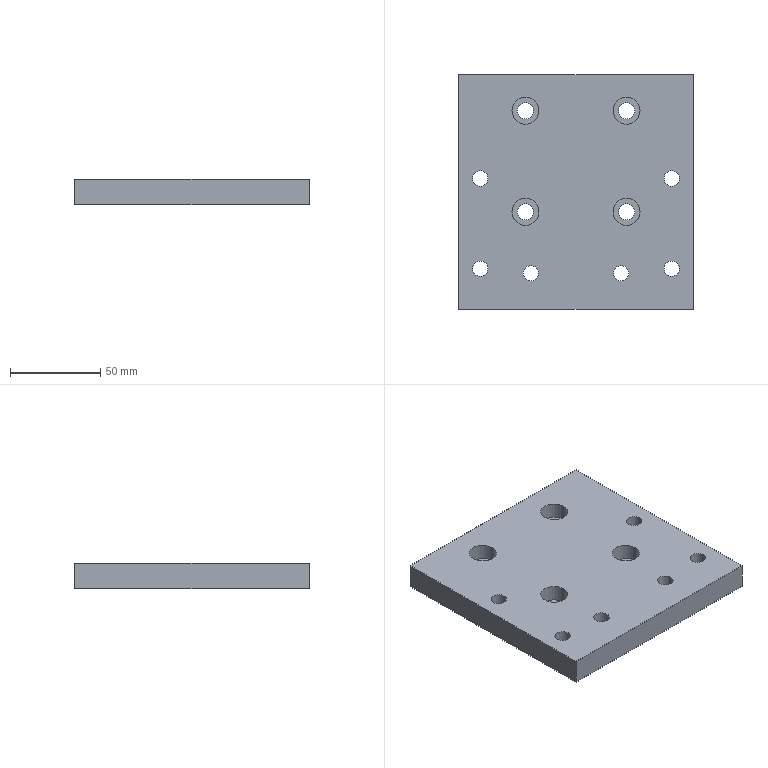Part | SolidWorks | features HoleWzd 3, Extrusion 1, ICE 1 | 1 solid | 38 faces | box 130 x 130 x 14 mm | volume 224199 mm3 | cylinder 28 | plane 10 | commonest cylinder face diameters 8.5 x12 9 x8 15 x8
STEP:
#1=CARTESIAN_POINT('',(122.25,72.5,14.));
#2=VERTEX_POINT('',#1);
#3=CARTESIAN_POINT('',(113.75,72.5,14.));
#4=VERTEX_POINT('',#3);
#5=CARTESIAN_POINT('',(118.,72.5,14.));
#6=DIRECTION('',(0.,0.,-1.));
#7=DIRECTION('',(-1.,0.,0.));
#8=AXIS2_PLACEMENT_3D('',#5,#6,#7);
#9=CIRCLE('',#8,4.25);
#10=EDGE_CURVE('',#2,#4,#9,.T.);
#11=ORIENTED_EDGE('',*,*,#10,.F.);
#12=CARTESIAN_POINT('',(122.25,72.5,0.));
#13=VERTEX_POINT('',#12);
#14=CARTESIAN_POINT('',(122.25,72.5,0.));
#15=DIRECTION('',(0.,0.,-1.));
#16=VECTOR('',#15,1000.);
#17=LINE('',#14,#16);
#18=EDGE_CURVE('',#2,#13,#17,.T.);
#19=ORIENTED_EDGE('',*,*,#18,.T.);
#20=CARTESIAN_POINT('',(113.75,72.5,0.));
#21=VERTEX_POINT('',#20);
#22=CARTESIAN_POINT('',(118.,72.5,0.));
#23=DIRECTION('',(0.,0.,-1.));
#24=DIRECTION('',(-1.,0.,0.));
#25=AXIS2_PLACEMENT_3D('',#22,#23,#24);
#26=CIRCLE('',#25,4.25);
#27=EDGE_CURVE('',#13,#21,#26,.T.);
#28=ORIENTED_EDGE('',*,*,#27,.T.);
#29=CARTESIAN_POINT('',(113.75,72.5,0.));
#30=DIRECTION('',(0.,0.,-1.));
#31=VECTOR('',#30,1000.);
#32=LINE('',#29,#31);
#33=EDGE_CURVE('',#4,#21,#32,.T.);
#34=ORIENTED_EDGE('',*,*,#33,.F.);
#35=EDGE_LOOP('',(#11,#19,#28,#34));
#36=FACE_OUTER_BOUND('',#35,.T.);
#37=CARTESIAN_POINT('',(118.,72.5,0.));
#38=DIRECTION('',(0.,0.,-1.));
#39=DIRECTION('',(-1.,0.,0.));
#40=AXIS2_PLACEMENT_3D('',#37,#38,#39);
#41=CYLINDRICAL_SURFACE('',#40,4.25);
#42=ADVANCED_FACE('',(#36),#41,.F.);
#43=CARTESIAN_POINT('',(122.25,22.5,14.));
#44=VERTEX_POINT('',#43);
#45=CARTESIAN_POINT('',(113.75,22.5,14.));
#46=VERTEX_POINT('',#45);
#47=CARTESIAN_POINT('',(118.,22.5,14.));
#48=DIRECTION('',(0.,0.,-1.));
#49=DIRECTION('',(-1.,0.,0.));
#50=AXIS2_PLACEMENT_3D('',#47,#48,#49);
#51=CIRCLE('',#50,4.25);
#52=EDGE_CURVE('',#44,#46,#51,.T.);
#53=ORIENTED_EDGE('',*,*,#52,.F.);
#54=CARTESIAN_POINT('',(122.25,22.5,0.));
#55=VERTEX_POINT('',#54);
#56=CARTESIAN_POINT('',(122.25,22.5,0.));
#57=DIRECTION('',(0.,0.,-1.));
#58=VECTOR('',#57,1000.);
#59=LINE('',#56,#58);
#60=EDGE_CURVE('',#44,#55,#59,.T.);
#61=ORIENTED_EDGE('',*,*,#60,.T.);
#62=CARTESIAN_POINT('',(113.75,22.5,0.));
#63=VERTEX_POINT('',#62);
#64=CARTESIAN_POINT('',(118.,22.5,0.));
#65=DIRECTION('',(0.,0.,-1.));
#66=DIRECTION('',(-1.,0.,0.));
#67=AXIS2_PLACEMENT_3D('',#64,#65,#66);
#68=CIRCLE('',#67,4.25);
#69=EDGE_CURVE('',#55,#63,#68,.T.);
#70=ORIENTED_EDGE('',*,*,#69,.T.);
#71=CARTESIAN_POINT('',(113.75,22.5,0.));
#72=DIRECTION('',(0.,0.,-1.));
#73=VECTOR('',#72,1000.);
#74=LINE('',#71,#73);
#75=EDGE_CURVE('',#46,#63,#74,.T.);
#76=ORIENTED_EDGE('',*,*,#75,.F.);
#77=EDGE_LOOP('',(#53,#61,#70,#76));
#78=FACE_OUTER_BOUND('',#77,.T.);
#79=CARTESIAN_POINT('',(118.,22.5,0.));
#80=DIRECTION('',(0.,0.,-1.));
#81=DIRECTION('',(-1.,0.,0.));
#82=AXIS2_PLACEMENT_3D('',#79,#80,#81);
#83=CYLINDRICAL_SURFACE('',#82,4.25);
#84=ADVANCED_FACE('',(#78),#83,.F.);
#85=CARTESIAN_POINT('',(16.25,72.5,14.));
#86=VERTEX_POINT('',#85);
#87=CARTESIAN_POINT('',(7.75,72.5,14.));
#88=VERTEX_POINT('',#87);
#89=CARTESIAN_POINT('',(12.,72.5,14.));
#90=DIRECTION('',(0.,0.,-1.));
#91=DIRECTION('',(-1.,0.,0.));
#92=AXIS2_PLACEMENT_3D('',#89,#90,#91);
#93=CIRCLE('',#92,4.25);
#94=EDGE_CURVE('',#86,#88,#93,.T.);
#95=ORIENTED_EDGE('',*,*,#94,.F.);
#96=CARTESIAN_POINT('',(16.25,72.5,0.));
#97=VERTEX_POINT('',#96);
#98=CARTESIAN_POINT('',(16.25,72.5,0.));
#99=DIRECTION('',(0.,0.,-1.));
#100=VECTOR('',#99,1000.);
#101=LINE('',#98,#100);
#102=EDGE_CURVE('',#86,#97,#101,.T.);
#103=ORIENTED_EDGE('',*,*,#102,.T.);
#104=CARTESIAN_POINT('',(7.75,72.5,0.));
#105=VERTEX_POINT('',#104);
#106=CARTESIAN_POINT('',(12.,72.5,0.));
#107=DIRECTION('',(0.,0.,-1.));
#108=DIRECTION('',(-1.,0.,0.));
#109=AXIS2_PLACEMENT_3D('',#106,#107,#108);
#110=CIRCLE('',#109,4.25);
#111=EDGE_CURVE('',#97,#105,#110,.T.);
#112=ORIENTED_EDGE('',*,*,#111,.T.);
#113=CARTESIAN_POINT('',(7.75,72.5,0.));
#114=DIRECTION('',(0.,0.,-1.));
#115=VECTOR('',#114,1000.);
#116=LINE('',#113,#115);
#117=EDGE_CURVE('',#88,#105,#116,.T.);
#118=ORIENTED_EDGE('',*,*,#117,.F.);
#119=EDGE_LOOP('',(#95,#103,#112,#118));
#120=FACE_OUTER_BOUND('',#119,.T.);
#121=CARTESIAN_POINT('',(12.,72.5,0.));
#122=DIRECTION('',(0.,0.,-1.));
#123=DIRECTION('',(-1.,0.,0.));
#124=AXIS2_PLACEMENT_3D('',#121,#122,#123);
#125=CYLINDRICAL_SURFACE('',#124,4.25);
#126=ADVANCED_FACE('',(#120),#125,.F.);
#127=CARTESIAN_POINT('',(16.25,22.5,14.));
#128=VERTEX_POINT('',#127);
#129=CARTESIAN_POINT('',(7.75,22.5,14.));
#130=VERTEX_POINT('',#129);
#131=CARTESIAN_POINT('',(12.,22.5,14.));
#132=DIRECTION('',(0.,0.,-1.));
#133=DIRECTION('',(-1.,0.,0.));
#134=AXIS2_PLACEMENT_3D('',#131,#132,#133);
#135=CIRCLE('',#134,4.25);
#136=EDGE_CURVE('',#128,#130,#135,.T.);
#137=ORIENTED_EDGE('',*,*,#136,.F.);
#138=CARTESIAN_POINT('',(16.25,22.5,0.));
#139=VERTEX_POINT('',#138);
#140=CARTESIAN_POINT('',(16.25,22.5,0.));
#141=DIRECTION('',(0.,0.,-1.));
#142=VECTOR('',#141,1000.);
#143=LINE('',#140,#142);
#144=EDGE_CURVE('',#128,#139,#143,.T.);
#145=ORIENTED_EDGE('',*,*,#144,.T.);
#146=CARTESIAN_POINT('',(7.75,22.5,0.));
#147=VERTEX_POINT('',#146);
#148=CARTESIAN_POINT('',(12.,22.5,0.));
#149=DIRECTION('',(0.,0.,-1.));
#150=DIRECTION('',(-1.,0.,0.));
#151=AXIS2_PLACEMENT_3D('',#148,#149,#150);
#152=CIRCLE('',#151,4.25);
#153=EDGE_CURVE('',#139,#147,#152,.T.);
#154=ORIENTED_EDGE('',*,*,#153,.T.);
#155=CARTESIAN_POINT('',(7.75,22.5,0.));
#156=DIRECTION('',(0.,0.,-1.));
#157=VECTOR('',#156,1000.);
#158=LINE('',#155,#157);
#159=EDGE_CURVE('',#130,#147,#158,.T.);
#160=ORIENTED_EDGE('',*,*,#159,.F.);
#161=EDGE_LOOP('',(#137,#145,#154,#160));
#162=FACE_OUTER_BOUND('',#161,.T.);
#163=CARTESIAN_POINT('',(12.,22.5,0.));
#164=DIRECTION('',(0.,0.,-1.));
#165=DIRECTION('',(-1.,0.,0.));
#166=AXIS2_PLACEMENT_3D('',#163,#164,#165);
#167=CYLINDRICAL_SURFACE('',#166,4.25);
#168=ADVANCED_FACE('',(#162),#167,.F.);
#169=CARTESIAN_POINT('',(94.25,20.,14.));
#170=VERTEX_POINT('',#169);
#171=CARTESIAN_POINT('',(85.75,20.,14.));
#172=VERTEX_POINT('',#171);
#173=CARTESIAN_POINT('',(90.,20.,14.));
#174=DIRECTION('',(0.,0.,-1.));
#175=DIRECTION('',(-1.,0.,0.));
#176=AXIS2_PLACEMENT_3D('',#173,#174,#175);
#177=CIRCLE('',#176,4.25);
#178=EDGE_CURVE('',#170,#172,#177,.T.);
#179=ORIENTED_EDGE('',*,*,#178,.F.);
#180=CARTESIAN_POINT('',(94.25,20.,0.));
#181=VERTEX_POINT('',#180);
#182=CARTESIAN_POINT('',(94.25,20.,0.));
#183=DIRECTION('',(0.,0.,-1.));
#184=VECTOR('',#183,1000.);
#185=LINE('',#182,#184);
#186=EDGE_CURVE('',#170,#181,#185,.T.);
#187=ORIENTED_EDGE('',*,*,#186,.T.);
#188=CARTESIAN_POINT('',(85.75,20.,0.));
#189=VERTEX_POINT('',#188);
#190=CARTESIAN_POINT('',(90.,20.,0.));
#191=DIRECTION('',(0.,0.,-1.));
#192=DIRECTION('',(-1.,0.,0.));
#193=AXIS2_PLACEMENT_3D('',#190,#191,#192);
#194=CIRCLE('',#193,4.25);
#195=EDGE_CURVE('',#181,#189,#194,.T.);
#196=ORIENTED_EDGE('',*,*,#195,.T.);
#197=CARTESIAN_POINT('',(85.75,20.,0.));
#198=DIRECTION('',(0.,0.,-1.));
#199=VECTOR('',#198,1000.);
#200=LINE('',#197,#199);
#201=EDGE_CURVE('',#172,#189,#200,.T.);
#202=ORIENTED_EDGE('',*,*,#201,.F.);
#203=EDGE_LOOP('',(#179,#187,#196,#202));
#204=FACE_OUTER_BOUND('',#203,.T.);
#205=CARTESIAN_POINT('',(90.,20.,0.));
#206=DIRECTION('',(0.,0.,-1.));
#207=DIRECTION('',(-1.,0.,0.));
#208=AXIS2_PLACEMENT_3D('',#205,#206,#207);
#209=CYLINDRICAL_SURFACE('',#208,4.25);
#210=ADVANCED_FACE('',(#204),#209,.F.);
#211=CARTESIAN_POINT('',(44.25,20.,14.));
#212=VERTEX_POINT('',#211);
#213=CARTESIAN_POINT('',(35.75,20.,14.));
#214=VERTEX_POINT('',#213);
#215=CARTESIAN_POINT('',(40.,20.,14.));
#216=DIRECTION('',(0.,0.,-1.));
#217=DIRECTION('',(-1.,0.,0.));
#218=AXIS2_PLACEMENT_3D('',#215,#216,#217);
#219=CIRCLE('',#218,4.25);
#220=EDGE_CURVE('',#212,#214,#219,.T.);
#221=ORIENTED_EDGE('',*,*,#220,.F.);
#222=CARTESIAN_POINT('',(44.25,20.,0.));
#223=VERTEX_POINT('',#222);
#224=CARTESIAN_POINT('',(44.25,20.,0.));
#225=DIRECTION('',(0.,0.,-1.));
#226=VECTOR('',#225,1000.);
#227=LINE('',#224,#226);
#228=EDGE_CURVE('',#212,#223,#227,.T.);
#229=ORIENTED_EDGE('',*,*,#228,.T.);
#230=CARTESIAN_POINT('',(35.75,20.,0.));
#231=VERTEX_POINT('',#230);
#232=CARTESIAN_POINT('',(40.,20.,0.));
#233=DIRECTION('',(0.,0.,-1.));
#234=DIRECTION('',(-1.,0.,0.));
#235=AXIS2_PLACEMENT_3D('',#232,#233,#234);
#236=CIRCLE('',#235,4.25);
#237=EDGE_CURVE('',#223,#231,#236,.T.);
#238=ORIENTED_EDGE('',*,*,#237,.T.);
#239=CARTESIAN_POINT('',(35.75,20.,0.));
#240=DIRECTION('',(0.,0.,-1.));
#241=VECTOR('',#240,1000.);
#242=LINE('',#239,#241);
#243=EDGE_CURVE('',#214,#231,#242,.T.);
#244=ORIENTED_EDGE('',*,*,#243,.F.);
#245=EDGE_LOOP('',(#221,#229,#238,#244));
#246=FACE_OUTER_BOUND('',#245,.T.);
#247=CARTESIAN_POINT('',(40.,20.,0.));
#248=DIRECTION('',(0.,0.,-1.));
#249=DIRECTION('',(-1.,0.,0.));
#250=AXIS2_PLACEMENT_3D('',#247,#248,#249);
#251=CYLINDRICAL_SURFACE('',#250,4.25);
#252=ADVANCED_FACE('',(#246),#251,.F.);
#253=CARTESIAN_POINT('',(29.5,110.,5.));
#254=VERTEX_POINT('',#253);
#255=CARTESIAN_POINT('',(44.5,110.,5.));
#256=VERTEX_POINT('',#255);
#257=CARTESIAN_POINT('',(37.,110.,5.));
#258=DIRECTION('',(0.,0.,1.));
#259=DIRECTION('',(1.,0.,0.));
#260=AXIS2_PLACEMENT_3D('',#257,#258,#259);
#261=CIRCLE('',#260,7.5);
#262=EDGE_CURVE('',#254,#256,#261,.T.);
#263=ORIENTED_EDGE('',*,*,#262,.F.);
#264=CARTESIAN_POINT('',(29.5,110.,14.));
#265=VERTEX_POINT('',#264);
#266=CARTESIAN_POINT('',(29.5,110.,14.));
#267=DIRECTION('',(0.,0.,1.));
#268=VECTOR('',#267,1000.);
#269=LINE('',#266,#268);
#270=EDGE_CURVE('',#254,#265,#269,.T.);
#271=ORIENTED_EDGE('',*,*,#270,.T.);
#272=CARTESIAN_POINT('',(44.5,110.,14.));
#273=VERTEX_POINT('',#272);
#274=CARTESIAN_POINT('',(37.,110.,14.));
#275=DIRECTION('',(0.,0.,1.));
#276=DIRECTION('',(1.,0.,0.));
#277=AXIS2_PLACEMENT_3D('',#274,#275,#276);
#278=CIRCLE('',#277,7.5);
#279=EDGE_CURVE('',#265,#273,#278,.T.);
#280=ORIENTED_EDGE('',*,*,#279,.T.);
#281=CARTESIAN_POINT('',(44.5,110.,14.));
#282=DIRECTION('',(0.,0.,1.));
#283=VECTOR('',#282,1000.);
#284=LINE('',#281,#283);
#285=EDGE_CURVE('',#256,#273,#284,.T.);
#286=ORIENTED_EDGE('',*,*,#285,.F.);
#287=EDGE_LOOP('',(#263,#271,#280,#286));
#288=FACE_OUTER_BOUND('',#287,.T.);
#289=CARTESIAN_POINT('',(37.,110.,14.));
#290=DIRECTION('',(0.,0.,1.));
#291=DIRECTION('',(1.,0.,0.));
#292=AXIS2_PLACEMENT_3D('',#289,#290,#291);
#293=CYLINDRICAL_SURFACE('',#292,7.5);
#294=ADVANCED_FACE('',(#288),#293,.F.);
#295=CARTESIAN_POINT('',(32.5,110.,0.));
#296=VERTEX_POINT('',#295);
#297=CARTESIAN_POINT('',(41.5,110.,0.));
#298=VERTEX_POINT('',#297);
#299=CARTESIAN_POINT('',(37.,110.,0.));
#300=DIRECTION('',(0.,0.,1.));
#301=DIRECTION('',(1.,0.,0.));
#302=AXIS2_PLACEMENT_3D('',#299,#300,#301);
#303=CIRCLE('',#302,4.5);
#304=EDGE_CURVE('',#296,#298,#303,.T.);
#305=ORIENTED_EDGE('',*,*,#304,.F.);
#306=CARTESIAN_POINT('',(32.5,110.,5.));
#307=VERTEX_POINT('',#306);
#308=CARTESIAN_POINT('',(32.5,110.,14.));
#309=DIRECTION('',(0.,0.,1.));
#310=VECTOR('',#309,1000.);
#311=LINE('',#308,#310);
#312=EDGE_CURVE('',#296,#307,#311,.T.);
#313=ORIENTED_EDGE('',*,*,#312,.T.);
#314=CARTESIAN_POINT('',(41.5,110.,5.));
#315=VERTEX_POINT('',#314);
#316=CARTESIAN_POINT('',(37.,110.,5.));
#317=DIRECTION('',(0.,0.,1.));
#318=DIRECTION('',(1.,0.,0.));
#319=AXIS2_PLACEMENT_3D('',#316,#317,#318);
#320=CIRCLE('',#319,4.5);
#321=EDGE_CURVE('',#307,#315,#320,.T.);
#322=ORIENTED_EDGE('',*,*,#321,.T.);
#323=CARTESIAN_POINT('',(41.5,110.,14.));
#324=DIRECTION('',(0.,0.,1.));
#325=VECTOR('',#324,1000.);
#326=LINE('',#323,#325);
#327=EDGE_CURVE('',#298,#315,#326,.T.);
#328=ORIENTED_EDGE('',*,*,#327,.F.);
#329=EDGE_LOOP('',(#305,#313,#322,#328));
#330=FACE_OUTER_BOUND('',#329,.T.);
#331=CARTESIAN_POINT('',(37.,110.,14.));
#332=DIRECTION('',(0.,0.,1.));
#333=DIRECTION('',(1.,0.,0.));
#334=AXIS2_PLACEMENT_3D('',#331,#332,#333);
#335=CYLINDRICAL_SURFACE('',#334,4.5);
#336=ADVANCED_FACE('',(#330),#335,.F.);
#337=CARTESIAN_POINT('',(85.5,110.,5.));
#338=VERTEX_POINT('',#337);
#339=CARTESIAN_POINT('',(100.5,110.,5.));
#340=VERTEX_POINT('',#339);
#341=CARTESIAN_POINT('',(93.,110.,5.));
#342=DIRECTION('',(0.,0.,1.));
#343=DIRECTION('',(1.,0.,0.));
#344=AXIS2_PLACEMENT_3D('',#341,#342,#343);
#345=CIRCLE('',#344,7.5);
#346=EDGE_CURVE('',#338,#340,#345,.T.);
#347=ORIENTED_EDGE('',*,*,#346,.F.);
#348=CARTESIAN_POINT('',(85.5,110.,14.));
#349=VERTEX_POINT('',#348);
#350=CARTESIAN_POINT('',(85.5,110.,14.));
#351=DIRECTION('',(0.,0.,1.));
#352=VECTOR('',#351,1000.);
#353=LINE('',#350,#352);
#354=EDGE_CURVE('',#338,#349,#353,.T.);
#355=ORIENTED_EDGE('',*,*,#354,.T.);
#356=CARTESIAN_POINT('',(100.5,110.,14.));
#357=VERTEX_POINT('',#356);
#358=CARTESIAN_POINT('',(93.,110.,14.));
#359=DIRECTION('',(0.,0.,1.));
#360=DIRECTION('',(1.,0.,0.));
#361=AXIS2_PLACEMENT_3D('',#358,#359,#360);
#362=CIRCLE('',#361,7.5);
#363=EDGE_CURVE('',#349,#357,#362,.T.);
#364=ORIENTED_EDGE('',*,*,#363,.T.);
#365=CARTESIAN_POINT('',(100.5,110.,14.));
#366=DIRECTION('',(0.,0.,1.));
#367=VECTOR('',#366,1000.);
#368=LINE('',#365,#367);
#369=EDGE_CURVE('',#340,#357,#368,.T.);
#370=ORIENTED_EDGE('',*,*,#369,.F.);
#371=EDGE_LOOP('',(#347,#355,#364,#370));
#372=FACE_OUTER_BOUND('',#371,.T.);
#373=CARTESIAN_POINT('',(93.,110.,14.));
#374=DIRECTION('',(0.,0.,1.));
#375=DIRECTION('',(1.,0.,0.));
#376=AXIS2_PLACEMENT_3D('',#373,#374,#375);
#377=CYLINDRICAL_SURFACE('',#376,7.5);
#378=ADVANCED_FACE('',(#372),#377,.F.);
#379=CARTESIAN_POINT('',(88.5,110.,0.));
#380=VERTEX_POINT('',#379);
#381=CARTESIAN_POINT('',(97.5,110.,0.));
#382=VERTEX_POINT('',#381);
#383=CARTESIAN_POINT('',(93.,110.,0.));
#384=DIRECTION('',(0.,0.,1.));
#385=DIRECTION('',(1.,0.,0.));
#386=AXIS2_PLACEMENT_3D('',#383,#384,#385);
#387=CIRCLE('',#386,4.5);
#388=EDGE_CURVE('',#380,#382,#387,.T.);
#389=ORIENTED_EDGE('',*,*,#388,.F.);
#390=CARTESIAN_POINT('',(88.5,110.,5.));
#391=VERTEX_POINT('',#390);
#392=CARTESIAN_POINT('',(88.5,110.,14.));
#393=DIRECTION('',(0.,0.,1.));
#394=VECTOR('',#393,1000.);
#395=LINE('',#392,#394);
#396=EDGE_CURVE('',#380,#391,#395,.T.);
#397=ORIENTED_EDGE('',*,*,#396,.T.);
#398=CARTESIAN_POINT('',(97.5,110.,5.));
#399=VERTEX_POINT('',#398);
#400=CARTESIAN_POINT('',(93.,110.,5.));
#401=DIRECTION('',(0.,0.,1.));
#402=DIRECTION('',(1.,0.,0.));
#403=AXIS2_PLACEMENT_3D('',#400,#401,#402);
#404=CIRCLE('',#403,4.5);
#405=EDGE_CURVE('',#391,#399,#404,.T.);
#406=ORIENTED_EDGE('',*,*,#405,.T.);
#407=CARTESIAN_POINT('',(97.5,110.,14.));
#408=DIRECTION('',(0.,0.,1.));
#409=VECTOR('',#408,1000.);
#410=LINE('',#407,#409);
#411=EDGE_CURVE('',#382,#399,#410,.T.);
#412=ORIENTED_EDGE('',*,*,#411,.F.);
#413=EDGE_LOOP('',(#389,#397,#406,#412));
#414=FACE_OUTER_BOUND('',#413,.T.);
#415=CARTESIAN_POINT('',(93.,110.,14.));
#416=DIRECTION('',(0.,0.,1.));
#417=DIRECTION('',(1.,0.,0.));
#418=AXIS2_PLACEMENT_3D('',#415,#416,#417);
#419=CYLINDRICAL_SURFACE('',#418,4.5);
#420=ADVANCED_FACE('',(#414),#419,.F.);
#421=CARTESIAN_POINT('',(85.5,54.,5.));
#422=VERTEX_POINT('',#421);
#423=CARTESIAN_POINT('',(100.5,54.,5.));
#424=VERTEX_POINT('',#423);
#425=CARTESIAN_POINT('',(93.,54.,5.));
#426=DIRECTION('',(0.,0.,1.));
#427=DIRECTION('',(1.,0.,0.));
#428=AXIS2_PLACEMENT_3D('',#425,#426,#427);
#429=CIRCLE('',#428,7.5);
#430=EDGE_CURVE('',#422,#424,#429,.T.);
#431=ORIENTED_EDGE('',*,*,#430,.F.);
#432=CARTESIAN_POINT('',(85.5,54.,14.));
#433=VERTEX_POINT('',#432);
#434=CARTESIAN_POINT('',(85.5,54.,14.));
#435=DIRECTION('',(0.,0.,1.));
#436=VECTOR('',#435,1000.);
#437=LINE('',#434,#436);
#438=EDGE_CURVE('',#422,#433,#437,.T.);
#439=ORIENTED_EDGE('',*,*,#438,.T.);
#440=CARTESIAN_POINT('',(100.5,54.,14.));
#441=VERTEX_POINT('',#440);
#442=CARTESIAN_POINT('',(93.,54.,14.));
#443=DIRECTION('',(0.,0.,1.));
#444=DIRECTION('',(1.,0.,0.));
#445=AXIS2_PLACEMENT_3D('',#442,#443,#444);
#446=CIRCLE('',#445,7.5);
#447=EDGE_CURVE('',#433,#441,#446,.T.);
#448=ORIENTED_EDGE('',*,*,#447,.T.);
#449=CARTESIAN_POINT('',(100.5,54.,14.));
#450=DIRECTION('',(0.,0.,1.));
#451=VECTOR('',#450,1000.);
#452=LINE('',#449,#451);
#453=EDGE_CURVE('',#424,#441,#452,.T.);
#454=ORIENTED_EDGE('',*,*,#453,.F.);
#455=EDGE_LOOP('',(#431,#439,#448,#454));
#456=FACE_OUTER_BOUND('',#455,.T.);
#457=CARTESIAN_POINT('',(93.,54.,14.));
#458=DIRECTION('',(0.,0.,1.));
#459=DIRECTION('',(1.,0.,0.));
#460=AXIS2_PLACEMENT_3D('',#457,#458,#459);
#461=CYLINDRICAL_SURFACE('',#460,7.5);
#462=ADVANCED_FACE('',(#456),#461,.F.);
#463=CARTESIAN_POINT('',(88.5,54.,0.));
#464=VERTEX_POINT('',#463);
#465=CARTESIAN_POINT('',(97.5,54.,0.));
#466=VERTEX_POINT('',#465);
#467=CARTESIAN_POINT('',(93.,54.,0.));
#468=DIRECTION('',(0.,0.,1.));
#469=DIRECTION('',(1.,0.,0.));
#470=AXIS2_PLACEMENT_3D('',#467,#468,#469);
#471=CIRCLE('',#470,4.5);
#472=EDGE_CURVE('',#464,#466,#471,.T.);
#473=ORIENTED_EDGE('',*,*,#472,.F.);
#474=CARTESIAN_POINT('',(88.5,54.,5.));
#475=VERTEX_POINT('',#474);
#476=CARTESIAN_POINT('',(88.5,54.,14.));
#477=DIRECTION('',(0.,0.,1.));
#478=VECTOR('',#477,1000.);
#479=LINE('',#476,#478);
#480=EDGE_CURVE('',#464,#475,#479,.T.);
#481=ORIENTED_EDGE('',*,*,#480,.T.);
#482=CARTESIAN_POINT('',(97.5,54.,5.));
#483=VERTEX_POINT('',#482);
#484=CARTESIAN_POINT('',(93.,54.,5.));
#485=DIRECTION('',(0.,0.,1.));
#486=DIRECTION('',(1.,0.,0.));
#487=AXIS2_PLACEMENT_3D('',#484,#485,#486);
#488=CIRCLE('',#487,4.5);
#489=EDGE_CURVE('',#475,#483,#488,.T.);
#490=ORIENTED_EDGE('',*,*,#489,.T.);
#491=CARTESIAN_POINT('',(97.5,54.,14.));
#492=DIRECTION('',(0.,0.,1.));
#493=VECTOR('',#492,1000.);
#494=LINE('',#491,#493);
#495=EDGE_CURVE('',#466,#483,#494,.T.);
#496=ORIENTED_EDGE('',*,*,#495,.F.);
#497=EDGE_LOOP('',(#473,#481,#490,#496));
#498=FACE_OUTER_BOUND('',#497,.T.);
#499=CARTESIAN_POINT('',(93.,54.,14.));
#500=DIRECTION('',(0.,0.,1.));
#501=DIRECTION('',(1.,0.,0.));
#502=AXIS2_PLACEMENT_3D('',#499,#500,#501);
#503=CYLINDRICAL_SURFACE('',#502,4.5);
#504=ADVANCED_FACE('',(#498),#503,.F.);
#505=CARTESIAN_POINT('',(29.5,54.,5.));
#506=VERTEX_POINT('',#505);
#507=CARTESIAN_POINT('',(44.5,54.,5.));
#508=VERTEX_POINT('',#507);
#509=CARTESIAN_POINT('',(37.,54.,5.));
#510=DIRECTION('',(0.,0.,1.));
#511=DIRECTION('',(1.,0.,0.));
#512=AXIS2_PLACEMENT_3D('',#509,#510,#511);
#513=CIRCLE('',#512,7.5);
#514=EDGE_CURVE('',#506,#508,#513,.T.);
#515=ORIENTED_EDGE('',*,*,#514,.F.);
#516=CARTESIAN_POINT('',(29.5,54.,14.));
#517=VERTEX_POINT('',#516);
#518=CARTESIAN_POINT('',(29.5,54.,14.));
#519=DIRECTION('',(0.,0.,1.));
#520=VECTOR('',#519,1000.);
#521=LINE('',#518,#520);
#522=EDGE_CURVE('',#506,#517,#521,.T.);
#523=ORIENTED_EDGE('',*,*,#522,.T.);
#524=CARTESIAN_POINT('',(44.5,54.,14.));
#525=VERTEX_POINT('',#524);
#526=CARTESIAN_POINT('',(37.,54.,14.));
#527=DIRECTION('',(0.,0.,1.));
#528=DIRECTION('',(1.,0.,0.));
#529=AXIS2_PLACEMENT_3D('',#526,#527,#528);
#530=CIRCLE('',#529,7.5);
#531=EDGE_CURVE('',#517,#525,#530,.T.);
#532=ORIENTED_EDGE('',*,*,#531,.T.);
#533=CARTESIAN_POINT('',(44.5,54.,14.));
#534=DIRECTION('',(0.,0.,1.));
#535=VECTOR('',#534,1000.);
#536=LINE('',#533,#535);
#537=EDGE_CURVE('',#508,#525,#536,.T.);
#538=ORIENTED_EDGE('',*,*,#537,.F.);
#539=EDGE_LOOP('',(#515,#523,#532,#538));
#540=FACE_OUTER_BOUND('',#539,.T.);
#541=CARTESIAN_POINT('',(37.,54.,14.));
#542=DIRECTION('',(0.,0.,1.));
#543=DIRECTION('',(1.,0.,0.));
#544=AXIS2_PLACEMENT_3D('',#541,#542,#543);
#545=CYLINDRICAL_SURFACE('',#544,7.5);
#546=ADVANCED_FACE('',(#540),#545,.F.);
#547=CARTESIAN_POINT('',(32.5,54.,0.));
#548=VERTEX_POINT('',#547);
#549=CARTESIAN_POINT('',(41.5,54.,0.));
#550=VERTEX_POINT('',#549);
#551=CARTESIAN_POINT('',(37.,54.,0.));
#552=DIRECTION('',(0.,0.,1.));
#553=DIRECTION('',(1.,0.,0.));
#554=AXIS2_PLACEMENT_3D('',#551,#552,#553);
#555=CIRCLE('',#554,4.5);
#556=EDGE_CURVE('',#548,#550,#555,.T.);
#557=ORIENTED_EDGE('',*,*,#556,.F.);
#558=CARTESIAN_POINT('',(32.5,54.,5.));
#559=VERTEX_POINT('',#558);
#560=CARTESIAN_POINT('',(32.5,54.,14.));
#561=DIRECTION('',(0.,0.,1.));
#562=VECTOR('',#561,1000.);
#563=LINE('',#560,#562);
#564=EDGE_CURVE('',#548,#559,#563,.T.);
#565=ORIENTED_EDGE('',*,*,#564,.T.);
#566=CARTESIAN_POINT('',(41.5,54.,5.));
#567=VERTEX_POINT('',#566);
#568=CARTESIAN_POINT('',(37.,54.,5.));
#569=DIRECTION('',(0.,0.,1.));
#570=DIRECTION('',(1.,0.,0.));
#571=AXIS2_PLACEMENT_3D('',#568,#569,#570);
#572=CIRCLE('',#571,4.5);
#573=EDGE_CURVE('',#559,#567,#572,.T.);
#574=ORIENTED_EDGE('',*,*,#573,.T.);
#575=CARTESIAN_POINT('',(41.5,54.,14.));
#576=DIRECTION('',(0.,0.,1.));
#577=VECTOR('',#576,1000.);
#578=LINE('',#575,#577);
#579=EDGE_CURVE('',#550,#567,#578,.T.);
#580=ORIENTED_EDGE('',*,*,#579,.F.);
#581=EDGE_LOOP('',(#557,#565,#574,#580));
#582=FACE_OUTER_BOUND('',#581,.T.);
#583=CARTESIAN_POINT('',(37.,54.,14.));
#584=DIRECTION('',(0.,0.,1.));
#585=DIRECTION('',(1.,0.,0.));
#586=AXIS2_PLACEMENT_3D('',#583,#584,#585);
#587=CYLINDRICAL_SURFACE('',#586,4.5);
#588=ADVANCED_FACE('',(#582),#587,.F.);
#589=CARTESIAN_POINT('',(0.,130.,0.));
#590=VERTEX_POINT('',#589);
#591=CARTESIAN_POINT('',(0.,0.,0.));
#592=VERTEX_POINT('',#591);
#593=CARTESIAN_POINT('',(0.,0.,0.));
#594=DIRECTION('',(0.,-1.,0.));
#595=VECTOR('',#594,1000.);
#596=LINE('',#593,#595);
#597=EDGE_CURVE('',#590,#592,#596,.T.);
#598=ORIENTED_EDGE('',*,*,#597,.T.);
#599=CARTESIAN_POINT('',(0.,0.,14.));
#600=VERTEX_POINT('',#599);
#601=CARTESIAN_POINT('',(0.,0.,14.));
#602=DIRECTION('',(0.,0.,-1.));
#603=VECTOR('',#602,1000.);
#604=LINE('',#601,#603);
#605=EDGE_CURVE('',#600,#592,#604,.T.);
#606=ORIENTED_EDGE('',*,*,#605,.F.);
#607=CARTESIAN_POINT('',(0.,130.,14.));
#608=VERTEX_POINT('',#607);
#609=CARTESIAN_POINT('',(0.,0.,14.));
#610=DIRECTION('',(0.,-1.,0.));
#611=VECTOR('',#610,1000.);
#612=LINE('',#609,#611);
#613=EDGE_CURVE('',#608,#600,#612,.T.);
#614=ORIENTED_EDGE('',*,*,#613,.F.);
#615=CARTESIAN_POINT('',(0.,130.,14.));
#616=DIRECTION('',(0.,0.,-1.));
#617=VECTOR('',#616,1000.);
#618=LINE('',#615,#617);
#619=EDGE_CURVE('',#608,#590,#618,.T.);
#620=ORIENTED_EDGE('',*,*,#619,.T.);
#621=EDGE_LOOP('',(#598,#606,#614,#620));
#622=FACE_OUTER_BOUND('',#621,.T.);
#623=CARTESIAN_POINT('',(0.,0.,14.));
#624=DIRECTION('',(1.,0.,0.));
#625=DIRECTION('',(0.,0.,-1.));
#626=AXIS2_PLACEMENT_3D('',#623,#624,#625);
#627=PLANE('',#626);
#628=ADVANCED_FACE('',(#622),#627,.F.);
#629=CARTESIAN_POINT('',(130.,0.,0.));
#630=VERTEX_POINT('',#629);
#631=CARTESIAN_POINT('',(0.,0.,0.));
#632=DIRECTION('',(1.,0.,0.));
#633=VECTOR('',#632,1000.);
#634=LINE('',#631,#633);
#635=EDGE_CURVE('',#592,#630,#634,.T.);
#636=ORIENTED_EDGE('',*,*,#635,.T.);
#637=CARTESIAN_POINT('',(130.,0.,14.));
#638=VERTEX_POINT('',#637);
#639=CARTESIAN_POINT('',(130.,0.,14.));
#640=DIRECTION('',(0.,0.,-1.));
#641=VECTOR('',#640,1000.);
#642=LINE('',#639,#641);
#643=EDGE_CURVE('',#638,#630,#642,.T.);
#644=ORIENTED_EDGE('',*,*,#643,.F.);
#645=CARTESIAN_POINT('',(0.,0.,14.));
#646=DIRECTION('',(1.,0.,0.));
#647=VECTOR('',#646,1000.);
#648=LINE('',#645,#647);
#649=EDGE_CURVE('',#600,#638,#648,.T.);
#650=ORIENTED_EDGE('',*,*,#649,.F.);
#651=ORIENTED_EDGE('',*,*,#605,.T.);
#652=EDGE_LOOP('',(#636,#644,#650,#651));
#653=FACE_OUTER_BOUND('',#652,.T.);
#654=CARTESIAN_POINT('',(0.,0.,14.));
#655=DIRECTION('',(0.,1.,0.));
#656=DIRECTION('',(0.,0.,1.));
#657=AXIS2_PLACEMENT_3D('',#654,#655,#656);
#658=PLANE('',#657);
#659=ADVANCED_FACE('',(#653),#658,.F.);
#660=CARTESIAN_POINT('',(130.,130.,0.));
#661=VERTEX_POINT('',#660);
#662=CARTESIAN_POINT('',(130.,0.,0.));
#663=DIRECTION('',(0.,1.,0.));
#664=VECTOR('',#663,1000.);
#665=LINE('',#662,#664);
#666=EDGE_CURVE('',#630,#661,#665,.T.);
#667=ORIENTED_EDGE('',*,*,#666,.T.);
#668=CARTESIAN_POINT('',(130.,130.,14.));
#669=VERTEX_POINT('',#668);
#670=CARTESIAN_POINT('',(130.,130.,14.));
#671=DIRECTION('',(0.,0.,-1.));
#672=VECTOR('',#671,1000.);
#673=LINE('',#670,#672);
#674=EDGE_CURVE('',#669,#661,#673,.T.);
#675=ORIENTED_EDGE('',*,*,#674,.F.);
#676=CARTESIAN_POINT('',(130.,0.,14.));
#677=DIRECTION('',(0.,1.,0.));
#678=VECTOR('',#677,1000.);
#679=LINE('',#676,#678);
#680=EDGE_CURVE('',#638,#669,#679,.T.);
#681=ORIENTED_EDGE('',*,*,#680,.F.);
#682=ORIENTED_EDGE('',*,*,#643,.T.);
#683=EDGE_LOOP('',(#667,#675,#681,#682));
#684=FACE_OUTER_BOUND('',#683,.T.);
#685=CARTESIAN_POINT('',(130.,0.,14.));
#686=DIRECTION('',(-1.,0.,0.));
#687=DIRECTION('',(0.,0.,1.));
#688=AXIS2_PLACEMENT_3D('',#685,#686,#687);
#689=PLANE('',#688);
#690=ADVANCED_FACE('',(#684),#689,.F.);
#691=CARTESIAN_POINT('',(0.,130.,0.));
#692=DIRECTION('',(-1.,0.,0.));
#693=VECTOR('',#692,1000.);
#694=LINE('',#691,#693);
#695=EDGE_CURVE('',#661,#590,#694,.T.);
#696=ORIENTED_EDGE('',*,*,#695,.T.);
#697=ORIENTED_EDGE('',*,*,#619,.F.);
#698=CARTESIAN_POINT('',(0.,130.,14.));
#699=DIRECTION('',(-1.,0.,0.));
#700=VECTOR('',#699,1000.);
#701=LINE('',#698,#700);
#702=EDGE_CURVE('',#669,#608,#701,.T.);
#703=ORIENTED_EDGE('',*,*,#702,.F.);
#704=ORIENTED_EDGE('',*,*,#674,.T.);
#705=EDGE_LOOP('',(#696,#697,#703,#704));
#706=FACE_OUTER_BOUND('',#705,.T.);
#707=CARTESIAN_POINT('',(0.,130.,14.));
#708=DIRECTION('',(0.,-1.,0.));
#709=DIRECTION('',(0.,0.,-1.));
#710=AXIS2_PLACEMENT_3D('',#707,#708,#709);
#711=PLANE('',#710);
#712=ADVANCED_FACE('',(#706),#711,.F.);
#713=CARTESIAN_POINT('',(118.,72.5,14.));
#714=DIRECTION('',(0.,0.,-1.));
#715=DIRECTION('',(-1.,0.,0.));
#716=AXIS2_PLACEMENT_3D('',#713,#714,#715);
#717=CIRCLE('',#716,4.25);
#718=EDGE_CURVE('',#4,#2,#717,.T.);
#719=ORIENTED_EDGE('',*,*,#718,.T.);
#720=ORIENTED_EDGE('',*,*,#10,.T.);
#721=EDGE_LOOP('',(#719,#720));
#722=FACE_BOUND('',#721,.T.);
#723=CARTESIAN_POINT('',(118.,22.5,14.));
#724=DIRECTION('',(0.,0.,-1.));
#725=DIRECTION('',(-1.,0.,0.));
#726=AXIS2_PLACEMENT_3D('',#723,#724,#725);
#727=CIRCLE('',#726,4.25);
#728=EDGE_CURVE('',#46,#44,#727,.T.);
#729=ORIENTED_EDGE('',*,*,#728,.T.);
#730=ORIENTED_EDGE('',*,*,#52,.T.);
#731=EDGE_LOOP('',(#729,#730));
#732=FACE_BOUND('',#731,.T.);
#733=CARTESIAN_POINT('',(12.,72.5,14.));
#734=DIRECTION('',(0.,0.,-1.));
#735=DIRECTION('',(-1.,0.,0.));
#736=AXIS2_PLACEMENT_3D('',#733,#734,#735);
#737=CIRCLE('',#736,4.25);
#738=EDGE_CURVE('',#88,#86,#737,.T.);
#739=ORIENTED_EDGE('',*,*,#738,.T.);
#740=ORIENTED_EDGE('',*,*,#94,.T.);
#741=EDGE_LOOP('',(#739,#740));
#742=FACE_BOUND('',#741,.T.);
#743=CARTESIAN_POINT('',(12.,22.5,14.));
#744=DIRECTION('',(0.,0.,-1.));
#745=DIRECTION('',(-1.,0.,0.));
#746=AXIS2_PLACEMENT_3D('',#743,#744,#745);
#747=CIRCLE('',#746,4.25);
#748=EDGE_CURVE('',#130,#128,#747,.T.);
#749=ORIENTED_EDGE('',*,*,#748,.T.);
#750=ORIENTED_EDGE('',*,*,#136,.T.);
#751=EDGE_LOOP('',(#749,#750));
#752=FACE_BOUND('',#751,.T.);
#753=CARTESIAN_POINT('',(90.,20.,14.));
#754=DIRECTION('',(0.,0.,-1.));
#755=DIRECTION('',(-1.,0.,0.));
#756=AXIS2_PLACEMENT_3D('',#753,#754,#755);
#757=CIRCLE('',#756,4.25);
#758=EDGE_CURVE('',#172,#170,#757,.T.);
#759=ORIENTED_EDGE('',*,*,#758,.T.);
#760=ORIENTED_EDGE('',*,*,#178,.T.);
#761=EDGE_LOOP('',(#759,#760));
#762=FACE_BOUND('',#761,.T.);
#763=CARTESIAN_POINT('',(40.,20.,14.));
#764=DIRECTION('',(0.,0.,-1.));
#765=DIRECTION('',(-1.,0.,0.));
#766=AXIS2_PLACEMENT_3D('',#763,#764,#765);
#767=CIRCLE('',#766,4.25);
#768=EDGE_CURVE('',#214,#212,#767,.T.);
#769=ORIENTED_EDGE('',*,*,#768,.T.);
#770=ORIENTED_EDGE('',*,*,#220,.T.);
#771=EDGE_LOOP('',(#769,#770));
#772=FACE_BOUND('',#771,.T.);
#773=CARTESIAN_POINT('',(37.,110.,14.));
#774=DIRECTION('',(0.,0.,1.));
#775=DIRECTION('',(1.,0.,0.));
#776=AXIS2_PLACEMENT_3D('',#773,#774,#775);
#777=CIRCLE('',#776,7.5);
#778=EDGE_CURVE('',#273,#265,#777,.T.);
#779=ORIENTED_EDGE('',*,*,#778,.F.);
#780=ORIENTED_EDGE('',*,*,#279,.F.);
#781=EDGE_LOOP('',(#779,#780));
#782=FACE_BOUND('',#781,.T.);
#783=CARTESIAN_POINT('',(93.,110.,14.));
#784=DIRECTION('',(0.,0.,1.));
#785=DIRECTION('',(1.,0.,0.));
#786=AXIS2_PLACEMENT_3D('',#783,#784,#785);
#787=CIRCLE('',#786,7.5);
#788=EDGE_CURVE('',#357,#349,#787,.T.);
#789=ORIENTED_EDGE('',*,*,#788,.F.);
#790=ORIENTED_EDGE('',*,*,#363,.F.);
#791=EDGE_LOOP('',(#789,#790));
#792=FACE_BOUND('',#791,.T.);
#793=CARTESIAN_POINT('',(93.,54.,14.));
#794=DIRECTION('',(0.,0.,1.));
#795=DIRECTION('',(1.,0.,0.));
#796=AXIS2_PLACEMENT_3D('',#793,#794,#795);
#797=CIRCLE('',#796,7.5);
#798=EDGE_CURVE('',#441,#433,#797,.T.);
#799=ORIENTED_EDGE('',*,*,#798,.F.);
#800=ORIENTED_EDGE('',*,*,#447,.F.);
#801=EDGE_LOOP('',(#799,#800));
#802=FACE_BOUND('',#801,.T.);
#803=CARTESIAN_POINT('',(37.,54.,14.));
#804=DIRECTION('',(0.,0.,1.));
#805=DIRECTION('',(1.,0.,0.));
#806=AXIS2_PLACEMENT_3D('',#803,#804,#805);
#807=CIRCLE('',#806,7.5);
#808=EDGE_CURVE('',#525,#517,#807,.T.);
#809=ORIENTED_EDGE('',*,*,#808,.F.);
#810=ORIENTED_EDGE('',*,*,#531,.F.);
#811=EDGE_LOOP('',(#809,#810));
#812=FACE_BOUND('',#811,.T.);
#813=ORIENTED_EDGE('',*,*,#613,.T.);
#814=ORIENTED_EDGE('',*,*,#649,.T.);
#815=ORIENTED_EDGE('',*,*,#680,.T.);
#816=ORIENTED_EDGE('',*,*,#702,.T.);
#817=EDGE_LOOP('',(#813,#814,#815,#816));
#818=FACE_OUTER_BOUND('',#817,.T.);
#819=CARTESIAN_POINT('',(0.,0.,14.));
#820=DIRECTION('',(0.,0.,-1.));
#821=DIRECTION('',(-1.,0.,0.));
#822=AXIS2_PLACEMENT_3D('',#819,#820,#821);
#823=PLANE('',#822);
#824=ADVANCED_FACE('',(#722,#732,#742,#752,#762,#772,#782,#792,#802,#812,#818),#823,.F.);
#825=CARTESIAN_POINT('',(118.,72.5,0.));
#826=DIRECTION('',(0.,0.,-1.));
#827=DIRECTION('',(-1.,0.,0.));
#828=AXIS2_PLACEMENT_3D('',#825,#826,#827);
#829=CIRCLE('',#828,4.25);
#830=EDGE_CURVE('',#21,#13,#829,.T.);
#831=ORIENTED_EDGE('',*,*,#830,.F.);
#832=ORIENTED_EDGE('',*,*,#27,.F.);
#833=EDGE_LOOP('',(#831,#832));
#834=FACE_BOUND('',#833,.T.);
#835=CARTESIAN_POINT('',(118.,22.5,0.));
#836=DIRECTION('',(0.,0.,-1.));
#837=DIRECTION('',(-1.,0.,0.));
#838=AXIS2_PLACEMENT_3D('',#835,#836,#837);
#839=CIRCLE('',#838,4.25);
#840=EDGE_CURVE('',#63,#55,#839,.T.);
#841=ORIENTED_EDGE('',*,*,#840,.F.);
#842=ORIENTED_EDGE('',*,*,#69,.F.);
#843=EDGE_LOOP('',(#841,#842));
#844=FACE_BOUND('',#843,.T.);
#845=CARTESIAN_POINT('',(12.,72.5,0.));
#846=DIRECTION('',(0.,0.,-1.));
#847=DIRECTION('',(-1.,0.,0.));
#848=AXIS2_PLACEMENT_3D('',#845,#846,#847);
#849=CIRCLE('',#848,4.25);
#850=EDGE_CURVE('',#105,#97,#849,.T.);
#851=ORIENTED_EDGE('',*,*,#850,.F.);
#852=ORIENTED_EDGE('',*,*,#111,.F.);
#853=EDGE_LOOP('',(#851,#852));
#854=FACE_BOUND('',#853,.T.);
#855=CARTESIAN_POINT('',(12.,22.5,0.));
#856=DIRECTION('',(0.,0.,-1.));
#857=DIRECTION('',(-1.,0.,0.));
#858=AXIS2_PLACEMENT_3D('',#855,#856,#857);
#859=CIRCLE('',#858,4.25);
#860=EDGE_CURVE('',#147,#139,#859,.T.);
#861=ORIENTED_EDGE('',*,*,#860,.F.);
#862=ORIENTED_EDGE('',*,*,#153,.F.);
#863=EDGE_LOOP('',(#861,#862));
#864=FACE_BOUND('',#863,.T.);
#865=CARTESIAN_POINT('',(90.,20.,0.));
#866=DIRECTION('',(0.,0.,-1.));
#867=DIRECTION('',(-1.,0.,0.));
#868=AXIS2_PLACEMENT_3D('',#865,#866,#867);
#869=CIRCLE('',#868,4.25);
#870=EDGE_CURVE('',#189,#181,#869,.T.);
#871=ORIENTED_EDGE('',*,*,#870,.F.);
#872=ORIENTED_EDGE('',*,*,#195,.F.);
#873=EDGE_LOOP('',(#871,#872));
#874=FACE_BOUND('',#873,.T.);
#875=CARTESIAN_POINT('',(40.,20.,0.));
#876=DIRECTION('',(0.,0.,-1.));
#877=DIRECTION('',(-1.,0.,0.));
#878=AXIS2_PLACEMENT_3D('',#875,#876,#877);
#879=CIRCLE('',#878,4.25);
#880=EDGE_CURVE('',#231,#223,#879,.T.);
#881=ORIENTED_EDGE('',*,*,#880,.F.);
#882=ORIENTED_EDGE('',*,*,#237,.F.);
#883=EDGE_LOOP('',(#881,#882));
#884=FACE_BOUND('',#883,.T.);
#885=CARTESIAN_POINT('',(37.,110.,0.));
#886=DIRECTION('',(0.,0.,1.));
#887=DIRECTION('',(1.,0.,0.));
#888=AXIS2_PLACEMENT_3D('',#885,#886,#887);
#889=CIRCLE('',#888,4.5);
#890=EDGE_CURVE('',#298,#296,#889,.T.);
#891=ORIENTED_EDGE('',*,*,#890,.T.);
#892=ORIENTED_EDGE('',*,*,#304,.T.);
#893=EDGE_LOOP('',(#891,#892));
#894=FACE_BOUND('',#893,.T.);
#895=CARTESIAN_POINT('',(93.,110.,0.));
#896=DIRECTION('',(0.,0.,1.));
#897=DIRECTION('',(1.,0.,0.));
#898=AXIS2_PLACEMENT_3D('',#895,#896,#897);
#899=CIRCLE('',#898,4.5);
#900=EDGE_CURVE('',#382,#380,#899,.T.);
#901=ORIENTED_EDGE('',*,*,#900,.T.);
#902=ORIENTED_EDGE('',*,*,#388,.T.);
#903=EDGE_LOOP('',(#901,#902));
#904=FACE_BOUND('',#903,.T.);
#905=CARTESIAN_POINT('',(93.,54.,0.));
#906=DIRECTION('',(0.,0.,1.));
#907=DIRECTION('',(1.,0.,0.));
#908=AXIS2_PLACEMENT_3D('',#905,#906,#907);
#909=CIRCLE('',#908,4.5);
#910=EDGE_CURVE('',#466,#464,#909,.T.);
#911=ORIENTED_EDGE('',*,*,#910,.T.);
#912=ORIENTED_EDGE('',*,*,#472,.T.);
#913=EDGE_LOOP('',(#911,#912));
#914=FACE_BOUND('',#913,.T.);
#915=CARTESIAN_POINT('',(37.,54.,0.));
#916=DIRECTION('',(0.,0.,1.));
#917=DIRECTION('',(1.,0.,0.));
#918=AXIS2_PLACEMENT_3D('',#915,#916,#917);
#919=CIRCLE('',#918,4.5);
#920=EDGE_CURVE('',#550,#548,#919,.T.);
#921=ORIENTED_EDGE('',*,*,#920,.T.);
#922=ORIENTED_EDGE('',*,*,#556,.T.);
#923=EDGE_LOOP('',(#921,#922));
#924=FACE_BOUND('',#923,.T.);
#925=ORIENTED_EDGE('',*,*,#597,.F.);
#926=ORIENTED_EDGE('',*,*,#695,.F.);
#927=ORIENTED_EDGE('',*,*,#666,.F.);
#928=ORIENTED_EDGE('',*,*,#635,.F.);
#929=EDGE_LOOP('',(#925,#926,#927,#928));
#930=FACE_OUTER_BOUND('',#929,.T.);
#931=CARTESIAN_POINT('',(0.,0.,0.));
#932=DIRECTION('',(0.,0.,-1.));
#933=DIRECTION('',(-1.,0.,0.));
#934=AXIS2_PLACEMENT_3D('',#931,#932,#933);
#935=PLANE('',#934);
#936=ADVANCED_FACE('',(#834,#844,#854,#864,#874,#884,#894,#904,#914,#924,#930),#935,.T.);
#937=ORIENTED_EDGE('',*,*,#564,.F.);
#938=ORIENTED_EDGE('',*,*,#920,.F.);
#939=ORIENTED_EDGE('',*,*,#579,.T.);
#940=CARTESIAN_POINT('',(37.,54.,5.));
#941=DIRECTION('',(0.,0.,1.));
#942=DIRECTION('',(1.,0.,0.));
#943=AXIS2_PLACEMENT_3D('',#940,#941,#942);
#944=CIRCLE('',#943,4.5);
#945=EDGE_CURVE('',#567,#559,#944,.T.);
#946=ORIENTED_EDGE('',*,*,#945,.T.);
#947=EDGE_LOOP('',(#937,#938,#939,#946));
#948=FACE_OUTER_BOUND('',#947,.T.);
#949=CARTESIAN_POINT('',(37.,54.,14.));
#950=DIRECTION('',(0.,0.,1.));
#951=DIRECTION('',(1.,0.,0.));
#952=AXIS2_PLACEMENT_3D('',#949,#950,#951);
#953=CYLINDRICAL_SURFACE('',#952,4.5);
#954=ADVANCED_FACE('',(#948),#953,.F.);
#955=ORIENTED_EDGE('',*,*,#945,.F.);
#956=ORIENTED_EDGE('',*,*,#573,.F.);
#957=EDGE_LOOP('',(#955,#956));
#958=FACE_BOUND('',#957,.T.);
#959=CARTESIAN_POINT('',(37.,54.,5.));
#960=DIRECTION('',(0.,0.,1.));
#961=DIRECTION('',(1.,0.,0.));
#962=AXIS2_PLACEMENT_3D('',#959,#960,#961);
#963=CIRCLE('',#962,7.5);
#964=EDGE_CURVE('',#508,#506,#963,.T.);
#965=ORIENTED_EDGE('',*,*,#964,.T.);
#966=ORIENTED_EDGE('',*,*,#514,.T.);
#967=EDGE_LOOP('',(#965,#966));
#968=FACE_OUTER_BOUND('',#967,.T.);
#969=CARTESIAN_POINT('',(41.5,54.,5.));
#970=DIRECTION('',(0.,0.,-1.));
#971=DIRECTION('',(-1.,0.,0.));
#972=AXIS2_PLACEMENT_3D('',#969,#970,#971);
#973=PLANE('',#972);
#974=ADVANCED_FACE('',(#958,#968),#973,.F.);
#975=ORIENTED_EDGE('',*,*,#522,.F.);
#976=ORIENTED_EDGE('',*,*,#964,.F.);
#977=ORIENTED_EDGE('',*,*,#537,.T.);
#978=ORIENTED_EDGE('',*,*,#808,.T.);
#979=EDGE_LOOP('',(#975,#976,#977,#978));
#980=FACE_OUTER_BOUND('',#979,.T.);
#981=CARTESIAN_POINT('',(37.,54.,14.));
#982=DIRECTION('',(0.,0.,1.));
#983=DIRECTION('',(1.,0.,0.));
#984=AXIS2_PLACEMENT_3D('',#981,#982,#983);
#985=CYLINDRICAL_SURFACE('',#984,7.5);
#986=ADVANCED_FACE('',(#980),#985,.F.);
#987=ORIENTED_EDGE('',*,*,#480,.F.);
#988=ORIENTED_EDGE('',*,*,#910,.F.);
#989=ORIENTED_EDGE('',*,*,#495,.T.);
#990=CARTESIAN_POINT('',(93.,54.,5.));
#991=DIRECTION('',(0.,0.,1.));
#992=DIRECTION('',(1.,0.,0.));
#993=AXIS2_PLACEMENT_3D('',#990,#991,#992);
#994=CIRCLE('',#993,4.5);
#995=EDGE_CURVE('',#483,#475,#994,.T.);
#996=ORIENTED_EDGE('',*,*,#995,.T.);
#997=EDGE_LOOP('',(#987,#988,#989,#996));
#998=FACE_OUTER_BOUND('',#997,.T.);
#999=CARTESIAN_POINT('',(93.,54.,14.));
#1000=DIRECTION('',(0.,0.,1.));
#1001=DIRECTION('',(1.,0.,0.));
#1002=AXIS2_PLACEMENT_3D('',#999,#1000,#1001);
#1003=CYLINDRICAL_SURFACE('',#1002,4.5);
#1004=ADVANCED_FACE('',(#998),#1003,.F.);
#1005=ORIENTED_EDGE('',*,*,#995,.F.);
#1006=ORIENTED_EDGE('',*,*,#489,.F.);
#1007=EDGE_LOOP('',(#1005,#1006));
#1008=FACE_BOUND('',#1007,.T.);
#1009=CARTESIAN_POINT('',(93.,54.,5.));
#1010=DIRECTION('',(0.,0.,1.));
#1011=DIRECTION('',(1.,0.,0.));
#1012=AXIS2_PLACEMENT_3D('',#1009,#1010,#1011);
#1013=CIRCLE('',#1012,7.5);
#1014=EDGE_CURVE('',#424,#422,#1013,.T.);
#1015=ORIENTED_EDGE('',*,*,#1014,.T.);
#1016=ORIENTED_EDGE('',*,*,#430,.T.);
#1017=EDGE_LOOP('',(#1015,#1016));
#1018=FACE_OUTER_BOUND('',#1017,.T.);
#1019=CARTESIAN_POINT('',(97.5,54.,5.));
#1020=DIRECTION('',(0.,0.,-1.));
#1021=DIRECTION('',(-1.,0.,0.));
#1022=AXIS2_PLACEMENT_3D('',#1019,#1020,#1021);
#1023=PLANE('',#1022);
#1024=ADVANCED_FACE('',(#1008,#1018),#1023,.F.);
#1025=ORIENTED_EDGE('',*,*,#438,.F.);
#1026=ORIENTED_EDGE('',*,*,#1014,.F.);
#1027=ORIENTED_EDGE('',*,*,#453,.T.);
#1028=ORIENTED_EDGE('',*,*,#798,.T.);
#1029=EDGE_LOOP('',(#1025,#1026,#1027,#1028));
#1030=FACE_OUTER_BOUND('',#1029,.T.);
#1031=CARTESIAN_POINT('',(93.,54.,14.));
#1032=DIRECTION('',(0.,0.,1.));
#1033=DIRECTION('',(1.,0.,0.));
#1034=AXIS2_PLACEMENT_3D('',#1031,#1032,#1033);
#1035=CYLINDRICAL_SURFACE('',#1034,7.5);
#1036=ADVANCED_FACE('',(#1030),#1035,.F.);
#1037=ORIENTED_EDGE('',*,*,#396,.F.);
#1038=ORIENTED_EDGE('',*,*,#900,.F.);
#1039=ORIENTED_EDGE('',*,*,#411,.T.);
#1040=CARTESIAN_POINT('',(93.,110.,5.));
#1041=DIRECTION('',(0.,0.,1.));
#1042=DIRECTION('',(1.,0.,0.));
#1043=AXIS2_PLACEMENT_3D('',#1040,#1041,#1042);
#1044=CIRCLE('',#1043,4.5);
#1045=EDGE_CURVE('',#399,#391,#1044,.T.);
#1046=ORIENTED_EDGE('',*,*,#1045,.T.);
#1047=EDGE_LOOP('',(#1037,#1038,#1039,#1046));
#1048=FACE_OUTER_BOUND('',#1047,.T.);
#1049=CARTESIAN_POINT('',(93.,110.,14.));
#1050=DIRECTION('',(0.,0.,1.));
#1051=DIRECTION('',(1.,0.,0.));
#1052=AXIS2_PLACEMENT_3D('',#1049,#1050,#1051);
#1053=CYLINDRICAL_SURFACE('',#1052,4.5);
#1054=ADVANCED_FACE('',(#1048),#1053,.F.);
#1055=ORIENTED_EDGE('',*,*,#1045,.F.);
#1056=ORIENTED_EDGE('',*,*,#405,.F.);
#1057=EDGE_LOOP('',(#1055,#1056));
#1058=FACE_BOUND('',#1057,.T.);
#1059=CARTESIAN_POINT('',(93.,110.,5.));
#1060=DIRECTION('',(0.,0.,1.));
#1061=DIRECTION('',(1.,0.,0.));
#1062=AXIS2_PLACEMENT_3D('',#1059,#1060,#1061);
#1063=CIRCLE('',#1062,7.5);
#1064=EDGE_CURVE('',#340,#338,#1063,.T.);
#1065=ORIENTED_EDGE('',*,*,#1064,.T.);
#1066=ORIENTED_EDGE('',*,*,#346,.T.);
#1067=EDGE_LOOP('',(#1065,#1066));
#1068=FACE_OUTER_BOUND('',#1067,.T.);
#1069=CARTESIAN_POINT('',(97.5,110.,5.));
#1070=DIRECTION('',(0.,0.,-1.));
#1071=DIRECTION('',(-1.,0.,0.));
#1072=AXIS2_PLACEMENT_3D('',#1069,#1070,#1071);
#1073=PLANE('',#1072);
#1074=ADVANCED_FACE('',(#1058,#1068),#1073,.F.);
#1075=ORIENTED_EDGE('',*,*,#354,.F.);
#1076=ORIENTED_EDGE('',*,*,#1064,.F.);
#1077=ORIENTED_EDGE('',*,*,#369,.T.);
#1078=ORIENTED_EDGE('',*,*,#788,.T.);
#1079=EDGE_LOOP('',(#1075,#1076,#1077,#1078));
#1080=FACE_OUTER_BOUND('',#1079,.T.);
#1081=CARTESIAN_POINT('',(93.,110.,14.));
#1082=DIRECTION('',(0.,0.,1.));
#1083=DIRECTION('',(1.,0.,0.));
#1084=AXIS2_PLACEMENT_3D('',#1081,#1082,#1083);
#1085=CYLINDRICAL_SURFACE('',#1084,7.5);
#1086=ADVANCED_FACE('',(#1080),#1085,.F.);
#1087=ORIENTED_EDGE('',*,*,#312,.F.);
#1088=ORIENTED_EDGE('',*,*,#890,.F.);
#1089=ORIENTED_EDGE('',*,*,#327,.T.);
#1090=CARTESIAN_POINT('',(37.,110.,5.));
#1091=DIRECTION('',(0.,0.,1.));
#1092=DIRECTION('',(1.,0.,0.));
#1093=AXIS2_PLACEMENT_3D('',#1090,#1091,#1092);
#1094=CIRCLE('',#1093,4.5);
#1095=EDGE_CURVE('',#315,#307,#1094,.T.);
#1096=ORIENTED_EDGE('',*,*,#1095,.T.);
#1097=EDGE_LOOP('',(#1087,#1088,#1089,#1096));
#1098=FACE_OUTER_BOUND('',#1097,.T.);
#1099=CARTESIAN_POINT('',(37.,110.,14.));
#1100=DIRECTION('',(0.,0.,1.));
#1101=DIRECTION('',(1.,0.,0.));
#1102=AXIS2_PLACEMENT_3D('',#1099,#1100,#1101);
#1103=CYLINDRICAL_SURFACE('',#1102,4.5);
#1104=ADVANCED_FACE('',(#1098),#1103,.F.);
#1105=ORIENTED_EDGE('',*,*,#1095,.F.);
#1106=ORIENTED_EDGE('',*,*,#321,.F.);
#1107=EDGE_LOOP('',(#1105,#1106));
#1108=FACE_BOUND('',#1107,.T.);
#1109=CARTESIAN_POINT('',(37.,110.,5.));
#1110=DIRECTION('',(0.,0.,1.));
#1111=DIRECTION('',(1.,0.,0.));
#1112=AXIS2_PLACEMENT_3D('',#1109,#1110,#1111);
#1113=CIRCLE('',#1112,7.5);
#1114=EDGE_CURVE('',#256,#254,#1113,.T.);
#1115=ORIENTED_EDGE('',*,*,#1114,.T.);
#1116=ORIENTED_EDGE('',*,*,#262,.T.);
#1117=EDGE_LOOP('',(#1115,#1116));
#1118=FACE_OUTER_BOUND('',#1117,.T.);
#1119=CARTESIAN_POINT('',(41.5,110.,5.));
#1120=DIRECTION('',(0.,0.,-1.));
#1121=DIRECTION('',(-1.,0.,0.));
#1122=AXIS2_PLACEMENT_3D('',#1119,#1120,#1121);
#1123=PLANE('',#1122);
#1124=ADVANCED_FACE('',(#1108,#1118),#1123,.F.);
#1125=ORIENTED_EDGE('',*,*,#270,.F.);
#1126=ORIENTED_EDGE('',*,*,#1114,.F.);
#1127=ORIENTED_EDGE('',*,*,#285,.T.);
#1128=ORIENTED_EDGE('',*,*,#778,.T.);
#1129=EDGE_LOOP('',(#1125,#1126,#1127,#1128));
#1130=FACE_OUTER_BOUND('',#1129,.T.);
#1131=CARTESIAN_POINT('',(37.,110.,14.));
#1132=DIRECTION('',(0.,0.,1.));
#1133=DIRECTION('',(1.,0.,0.));
#1134=AXIS2_PLACEMENT_3D('',#1131,#1132,#1133);
#1135=CYLINDRICAL_SURFACE('',#1134,7.5);
#1136=ADVANCED_FACE('',(#1130),#1135,.F.);
#1137=ORIENTED_EDGE('',*,*,#228,.F.);
#1138=ORIENTED_EDGE('',*,*,#768,.F.);
#1139=ORIENTED_EDGE('',*,*,#243,.T.);
#1140=ORIENTED_EDGE('',*,*,#880,.T.);
#1141=EDGE_LOOP('',(#1137,#1138,#1139,#1140));
#1142=FACE_OUTER_BOUND('',#1141,.T.);
#1143=CARTESIAN_POINT('',(40.,20.,0.));
#1144=DIRECTION('',(0.,0.,-1.));
#1145=DIRECTION('',(-1.,0.,0.));
#1146=AXIS2_PLACEMENT_3D('',#1143,#1144,#1145);
#1147=CYLINDRICAL_SURFACE('',#1146,4.25);
#1148=ADVANCED_FACE('',(#1142),#1147,.F.);
#1149=ORIENTED_EDGE('',*,*,#186,.F.);
#1150=ORIENTED_EDGE('',*,*,#758,.F.);
#1151=ORIENTED_EDGE('',*,*,#201,.T.);
#1152=ORIENTED_EDGE('',*,*,#870,.T.);
#1153=EDGE_LOOP('',(#1149,#1150,#1151,#1152));
#1154=FACE_OUTER_BOUND('',#1153,.T.);
#1155=CARTESIAN_POINT('',(90.,20.,0.));
#1156=DIRECTION('',(0.,0.,-1.));
#1157=DIRECTION('',(-1.,0.,0.));
#1158=AXIS2_PLACEMENT_3D('',#1155,#1156,#1157);
#1159=CYLINDRICAL_SURFACE('',#1158,4.25);
#1160=ADVANCED_FACE('',(#1154),#1159,.F.);
#1161=ORIENTED_EDGE('',*,*,#144,.F.);
#1162=ORIENTED_EDGE('',*,*,#748,.F.);
#1163=ORIENTED_EDGE('',*,*,#159,.T.);
#1164=ORIENTED_EDGE('',*,*,#860,.T.);
#1165=EDGE_LOOP('',(#1161,#1162,#1163,#1164));
#1166=FACE_OUTER_BOUND('',#1165,.T.);
#1167=CARTESIAN_POINT('',(12.,22.5,0.));
#1168=DIRECTION('',(0.,0.,-1.));
#1169=DIRECTION('',(-1.,0.,0.));
#1170=AXIS2_PLACEMENT_3D('',#1167,#1168,#1169);
#1171=CYLINDRICAL_SURFACE('',#1170,4.25);
#1172=ADVANCED_FACE('',(#1166),#1171,.F.);
#1173=ORIENTED_EDGE('',*,*,#102,.F.);
#1174=ORIENTED_EDGE('',*,*,#738,.F.);
#1175=ORIENTED_EDGE('',*,*,#117,.T.);
#1176=ORIENTED_EDGE('',*,*,#850,.T.);
#1177=EDGE_LOOP('',(#1173,#1174,#1175,#1176));
#1178=FACE_OUTER_BOUND('',#1177,.T.);
#1179=CARTESIAN_POINT('',(12.,72.5,0.));
#1180=DIRECTION('',(0.,0.,-1.));
#1181=DIRECTION('',(-1.,0.,0.));
#1182=AXIS2_PLACEMENT_3D('',#1179,#1180,#1181);
#1183=CYLINDRICAL_SURFACE('',#1182,4.25);
#1184=ADVANCED_FACE('',(#1178),#1183,.F.);
#1185=ORIENTED_EDGE('',*,*,#60,.F.);
#1186=ORIENTED_EDGE('',*,*,#728,.F.);
#1187=ORIENTED_EDGE('',*,*,#75,.T.);
#1188=ORIENTED_EDGE('',*,*,#840,.T.);
#1189=EDGE_LOOP('',(#1185,#1186,#1187,#1188));
#1190=FACE_OUTER_BOUND('',#1189,.T.);
#1191=CARTESIAN_POINT('',(118.,22.5,0.));
#1192=DIRECTION('',(0.,0.,-1.));
#1193=DIRECTION('',(-1.,0.,0.));
#1194=AXIS2_PLACEMENT_3D('',#1191,#1192,#1193);
#1195=CYLINDRICAL_SURFACE('',#1194,4.25);
#1196=ADVANCED_FACE('',(#1190),#1195,.F.);
#1197=ORIENTED_EDGE('',*,*,#18,.F.);
#1198=ORIENTED_EDGE('',*,*,#718,.F.);
#1199=ORIENTED_EDGE('',*,*,#33,.T.);
#1200=ORIENTED_EDGE('',*,*,#830,.T.);
#1201=EDGE_LOOP('',(#1197,#1198,#1199,#1200));
#1202=FACE_OUTER_BOUND('',#1201,.T.);
#1203=CARTESIAN_POINT('',(118.,72.5,0.));
#1204=DIRECTION('',(0.,0.,-1.));
#1205=DIRECTION('',(-1.,0.,0.));
#1206=AXIS2_PLACEMENT_3D('',#1203,#1204,#1205);
#1207=CYLINDRICAL_SURFACE('',#1206,4.25);
#1208=ADVANCED_FACE('',(#1202),#1207,.F.);
#1209=CLOSED_SHELL('',(#42,#84,#126,#168,#210,#252,#294,#336,#378,#420,#462,#504,#546,#588,#628,#659,#690,#712,#824,#936,#954,#974,#986,#1004,#1024,#1036,#1054,#1074,#1086,#1104,#1124,#1136,#1148,#1160,#1172,#1184,#1196,#1208));
#1210=MANIFOLD_SOLID_BREP('',#1209);
#1211=CARTESIAN_POINT('',(0.,0.,0.));
#1212=DIRECTION('',(0.,0.,1.));
#1213=DIRECTION('',(1.,0.,0.));
#1214=AXIS2_PLACEMENT_3D('',#1211,#1212,#1213);
#1215=(LENGTH_UNIT()NAMED_UNIT(*)SI_UNIT(.MILLI.,.METRE.));
#1216=UNCERTAINTY_MEASURE_WITH_UNIT(LENGTH_MEASURE(0.00001),#1215,'','');
#1217=(NAMED_UNIT(*)PLANE_ANGLE_UNIT()SI_UNIT($,.RADIAN.));
#1218=(NAMED_UNIT(*)SI_UNIT($,.STERADIAN.)SOLID_ANGLE_UNIT());
#1219=(GEOMETRIC_REPRESENTATION_CONTEXT(3)GLOBAL_UNCERTAINTY_ASSIGNED_CONTEXT((#1216))GLOBAL_UNIT_ASSIGNED_CONTEXT((#1215,#1217,#1218))REPRESENTATION_CONTEXT('',''));
#1220=ADVANCED_BREP_SHAPE_REPRESENTATION('',(#1210,#1214),#1219);